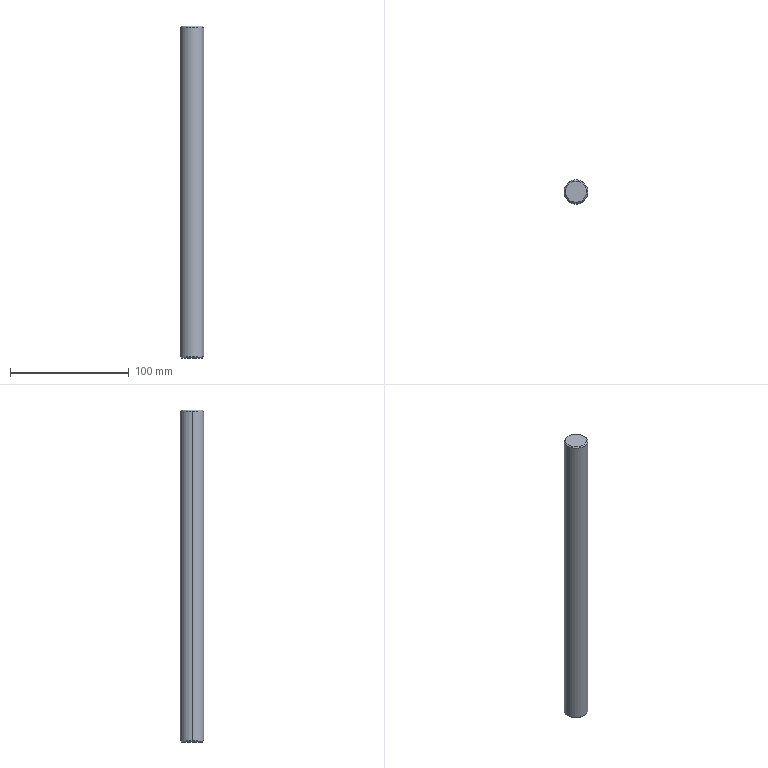Part | STEP file | Guide post | 1 solid | 8 faces | box 20 x 20 x 280 mm | volume 87904 mm3 | cone 4 | cylinder 2 | plane 2 | commonest cylinder face diameters 20 x2
STEP:
#1=CARTESIAN_POINT('',(59.373,-48.431,607.5));
#2=VERTEX_POINT('',#1);
#3=CARTESIAN_POINT('',(41.373,-48.431,607.5));
#4=VERTEX_POINT('',#3);
#5=CARTESIAN_POINT('',(50.373,-48.431,607.5));
#6=DIRECTION('',(0.,0.,1.));
#7=DIRECTION('',(-1.,0.,0.));
#8=AXIS2_PLACEMENT_3D('',#5,#6,#7);
#9=CIRCLE('',#8,9.);
#10=EDGE_CURVE('',#2,#4,#9,.T.);
#11=ORIENTED_EDGE('',*,*,#10,.F.);
#12=CARTESIAN_POINT('',(60.373,-48.431,606.5));
#13=VERTEX_POINT('',#12);
#14=CARTESIAN_POINT('',(60.373,-48.431,606.5));
#15=DIRECTION('',(0.7071,0.,-0.7071));
#16=VECTOR('',#15,1000.);
#17=LINE('',#14,#16);
#18=EDGE_CURVE('',#2,#13,#17,.T.);
#19=ORIENTED_EDGE('',*,*,#18,.T.);
#20=CARTESIAN_POINT('',(40.373,-48.431,606.5));
#21=VERTEX_POINT('',#20);
#22=CARTESIAN_POINT('',(50.373,-48.431,606.5));
#23=DIRECTION('',(0.,0.,-1.));
#24=DIRECTION('',(-1.,0.,0.));
#25=AXIS2_PLACEMENT_3D('',#22,#23,#24);
#26=CIRCLE('',#25,10.);
#27=EDGE_CURVE('',#21,#13,#26,.T.);
#28=ORIENTED_EDGE('',*,*,#27,.F.);
#29=CARTESIAN_POINT('',(40.373,-48.431,606.5));
#30=DIRECTION('',(-0.7071,0.,-0.7071));
#31=VECTOR('',#30,1000.);
#32=LINE('',#29,#31);
#33=EDGE_CURVE('',#4,#21,#32,.T.);
#34=ORIENTED_EDGE('',*,*,#33,.F.);
#35=EDGE_LOOP('',(#11,#19,#28,#34));
#36=FACE_OUTER_BOUND('',#35,.T.);
#37=CARTESIAN_POINT('',(50.373,-48.431,606.5));
#38=DIRECTION('',(0.,0.,-1.));
#39=DIRECTION('',(-1.,0.,0.));
#40=AXIS2_PLACEMENT_3D('',#37,#38,#39);
#41=CONICAL_SURFACE('',#40,10.,0.7854);
#42=ADVANCED_FACE('',(#36),#41,.T.);
#43=CARTESIAN_POINT('',(41.373,-48.431,327.5));
#44=VERTEX_POINT('',#43);
#45=CARTESIAN_POINT('',(59.373,-48.431,327.5));
#46=VERTEX_POINT('',#45);
#47=CARTESIAN_POINT('',(50.373,-48.431,327.5));
#48=DIRECTION('',(0.,0.,-1.));
#49=DIRECTION('',(-1.,0.,0.));
#50=AXIS2_PLACEMENT_3D('',#47,#48,#49);
#51=CIRCLE('',#50,9.);
#52=EDGE_CURVE('',#44,#46,#51,.T.);
#53=ORIENTED_EDGE('',*,*,#52,.F.);
#54=CARTESIAN_POINT('',(40.373,-48.431,328.5));
#55=VERTEX_POINT('',#54);
#56=CARTESIAN_POINT('',(41.373,-48.431,327.5));
#57=DIRECTION('',(-0.7071,0.,0.7071));
#58=VECTOR('',#57,1000.);
#59=LINE('',#56,#58);
#60=EDGE_CURVE('',#44,#55,#59,.T.);
#61=ORIENTED_EDGE('',*,*,#60,.T.);
#62=CARTESIAN_POINT('',(60.373,-48.431,328.5));
#63=VERTEX_POINT('',#62);
#64=CARTESIAN_POINT('',(50.373,-48.431,328.5));
#65=DIRECTION('',(0.,0.,1.));
#66=DIRECTION('',(-1.,0.,0.));
#67=AXIS2_PLACEMENT_3D('',#64,#65,#66);
#68=CIRCLE('',#67,10.);
#69=EDGE_CURVE('',#63,#55,#68,.T.);
#70=ORIENTED_EDGE('',*,*,#69,.F.);
#71=CARTESIAN_POINT('',(59.373,-48.431,327.5));
#72=DIRECTION('',(0.7071,0.,0.7071));
#73=VECTOR('',#72,1000.);
#74=LINE('',#71,#73);
#75=EDGE_CURVE('',#46,#63,#74,.T.);
#76=ORIENTED_EDGE('',*,*,#75,.F.);
#77=EDGE_LOOP('',(#53,#61,#70,#76));
#78=FACE_OUTER_BOUND('',#77,.T.);
#79=CARTESIAN_POINT('',(50.373,-48.431,327.5));
#80=DIRECTION('',(0.,0.,1.));
#81=DIRECTION('',(1.,0.,0.));
#82=AXIS2_PLACEMENT_3D('',#79,#80,#81);
#83=CONICAL_SURFACE('',#82,9.,0.7854);
#84=ADVANCED_FACE('',(#78),#83,.T.);
#85=ORIENTED_EDGE('',*,*,#69,.T.);
#86=CARTESIAN_POINT('',(40.373,-48.431,327.5));
#87=DIRECTION('',(0.,0.,1.));
#88=VECTOR('',#87,1000.);
#89=LINE('',#86,#88);
#90=EDGE_CURVE('',#55,#21,#89,.T.);
#91=ORIENTED_EDGE('',*,*,#90,.T.);
#92=ORIENTED_EDGE('',*,*,#27,.T.);
#93=CARTESIAN_POINT('',(60.373,-48.431,327.5));
#94=DIRECTION('',(0.,0.,1.));
#95=VECTOR('',#94,1000.);
#96=LINE('',#93,#95);
#97=EDGE_CURVE('',#63,#13,#96,.T.);
#98=ORIENTED_EDGE('',*,*,#97,.F.);
#99=EDGE_LOOP('',(#85,#91,#92,#98));
#100=FACE_OUTER_BOUND('',#99,.T.);
#101=CARTESIAN_POINT('',(50.373,-48.431,327.5));
#102=DIRECTION('',(0.,0.,1.));
#103=DIRECTION('',(1.,0.,0.));
#104=AXIS2_PLACEMENT_3D('',#101,#102,#103);
#105=CYLINDRICAL_SURFACE('',#104,10.);
#106=ADVANCED_FACE('',(#100),#105,.T.);
#107=ORIENTED_EDGE('',*,*,#90,.F.);
#108=CARTESIAN_POINT('',(50.373,-48.431,328.5));
#109=DIRECTION('',(0.,0.,1.));
#110=DIRECTION('',(-1.,0.,0.));
#111=AXIS2_PLACEMENT_3D('',#108,#109,#110);
#112=CIRCLE('',#111,10.);
#113=EDGE_CURVE('',#55,#63,#112,.T.);
#114=ORIENTED_EDGE('',*,*,#113,.T.);
#115=ORIENTED_EDGE('',*,*,#97,.T.);
#116=CARTESIAN_POINT('',(50.373,-48.431,606.5));
#117=DIRECTION('',(0.,0.,-1.));
#118=DIRECTION('',(-1.,0.,0.));
#119=AXIS2_PLACEMENT_3D('',#116,#117,#118);
#120=CIRCLE('',#119,10.);
#121=EDGE_CURVE('',#13,#21,#120,.T.);
#122=ORIENTED_EDGE('',*,*,#121,.T.);
#123=EDGE_LOOP('',(#107,#114,#115,#122));
#124=FACE_OUTER_BOUND('',#123,.T.);
#125=CARTESIAN_POINT('',(50.373,-48.431,327.5));
#126=DIRECTION('',(0.,0.,1.));
#127=DIRECTION('',(1.,0.,0.));
#128=AXIS2_PLACEMENT_3D('',#125,#126,#127);
#129=CYLINDRICAL_SURFACE('',#128,10.);
#130=ADVANCED_FACE('',(#124),#129,.T.);
#131=CARTESIAN_POINT('',(50.373,-48.431,327.5));
#132=DIRECTION('',(0.,0.,-1.));
#133=DIRECTION('',(-1.,0.,0.));
#134=AXIS2_PLACEMENT_3D('',#131,#132,#133);
#135=CIRCLE('',#134,9.);
#136=EDGE_CURVE('',#46,#44,#135,.T.);
#137=ORIENTED_EDGE('',*,*,#136,.T.);
#138=ORIENTED_EDGE('',*,*,#52,.T.);
#139=EDGE_LOOP('',(#137,#138));
#140=FACE_OUTER_BOUND('',#139,.T.);
#141=CARTESIAN_POINT('',(50.373,-48.431,327.5));
#142=DIRECTION('',(0.,0.,-1.));
#143=DIRECTION('',(-1.,0.,0.));
#144=AXIS2_PLACEMENT_3D('',#141,#142,#143);
#145=PLANE('',#144);
#146=ADVANCED_FACE('',(#140),#145,.T.);
#147=CARTESIAN_POINT('',(50.373,-48.431,607.5));
#148=DIRECTION('',(0.,0.,1.));
#149=DIRECTION('',(-1.,0.,0.));
#150=AXIS2_PLACEMENT_3D('',#147,#148,#149);
#151=CIRCLE('',#150,9.);
#152=EDGE_CURVE('',#4,#2,#151,.T.);
#153=ORIENTED_EDGE('',*,*,#152,.T.);
#154=ORIENTED_EDGE('',*,*,#10,.T.);
#155=EDGE_LOOP('',(#153,#154));
#156=FACE_OUTER_BOUND('',#155,.T.);
#157=CARTESIAN_POINT('',(50.373,-48.431,607.5));
#158=DIRECTION('',(0.,0.,-1.));
#159=DIRECTION('',(-1.,0.,0.));
#160=AXIS2_PLACEMENT_3D('',#157,#158,#159);
#161=PLANE('',#160);
#162=ADVANCED_FACE('',(#156),#161,.F.);
#163=ORIENTED_EDGE('',*,*,#60,.F.);
#164=ORIENTED_EDGE('',*,*,#136,.F.);
#165=ORIENTED_EDGE('',*,*,#75,.T.);
#166=ORIENTED_EDGE('',*,*,#113,.F.);
#167=EDGE_LOOP('',(#163,#164,#165,#166));
#168=FACE_OUTER_BOUND('',#167,.T.);
#169=CARTESIAN_POINT('',(50.373,-48.431,327.5));
#170=DIRECTION('',(0.,0.,1.));
#171=DIRECTION('',(1.,0.,0.));
#172=AXIS2_PLACEMENT_3D('',#169,#170,#171);
#173=CONICAL_SURFACE('',#172,9.,0.7854);
#174=ADVANCED_FACE('',(#168),#173,.T.);
#175=ORIENTED_EDGE('',*,*,#18,.F.);
#176=ORIENTED_EDGE('',*,*,#152,.F.);
#177=ORIENTED_EDGE('',*,*,#33,.T.);
#178=ORIENTED_EDGE('',*,*,#121,.F.);
#179=EDGE_LOOP('',(#175,#176,#177,#178));
#180=FACE_OUTER_BOUND('',#179,.T.);
#181=CARTESIAN_POINT('',(50.373,-48.431,606.5));
#182=DIRECTION('',(0.,0.,-1.));
#183=DIRECTION('',(-1.,0.,0.));
#184=AXIS2_PLACEMENT_3D('',#181,#182,#183);
#185=CONICAL_SURFACE('',#184,10.,0.7854);
#186=ADVANCED_FACE('',(#180),#185,.T.);
#187=CLOSED_SHELL('',(#42,#84,#106,#130,#146,#162,#174,#186));
#188=MANIFOLD_SOLID_BREP('',#187);
#189=CARTESIAN_POINT('',(0.,0.,0.));
#190=DIRECTION('',(0.,0.,1.));
#191=DIRECTION('',(1.,0.,0.));
#192=AXIS2_PLACEMENT_3D('',#189,#190,#191);
#193=(LENGTH_UNIT()NAMED_UNIT(*)SI_UNIT(.MILLI.,.METRE.));
#194=UNCERTAINTY_MEASURE_WITH_UNIT(LENGTH_MEASURE(0.00001),#193,'','');
#195=(NAMED_UNIT(*)PLANE_ANGLE_UNIT()SI_UNIT($,.RADIAN.));
#196=(NAMED_UNIT(*)SI_UNIT($,.STERADIAN.)SOLID_ANGLE_UNIT());
#197=(GEOMETRIC_REPRESENTATION_CONTEXT(3)GLOBAL_UNCERTAINTY_ASSIGNED_CONTEXT((#194))GLOBAL_UNIT_ASSIGNED_CONTEXT((#193,#195,#196))REPRESENTATION_CONTEXT('',''));
#198=ADVANCED_BREP_SHAPE_REPRESENTATION('',(#188,#192),#197);